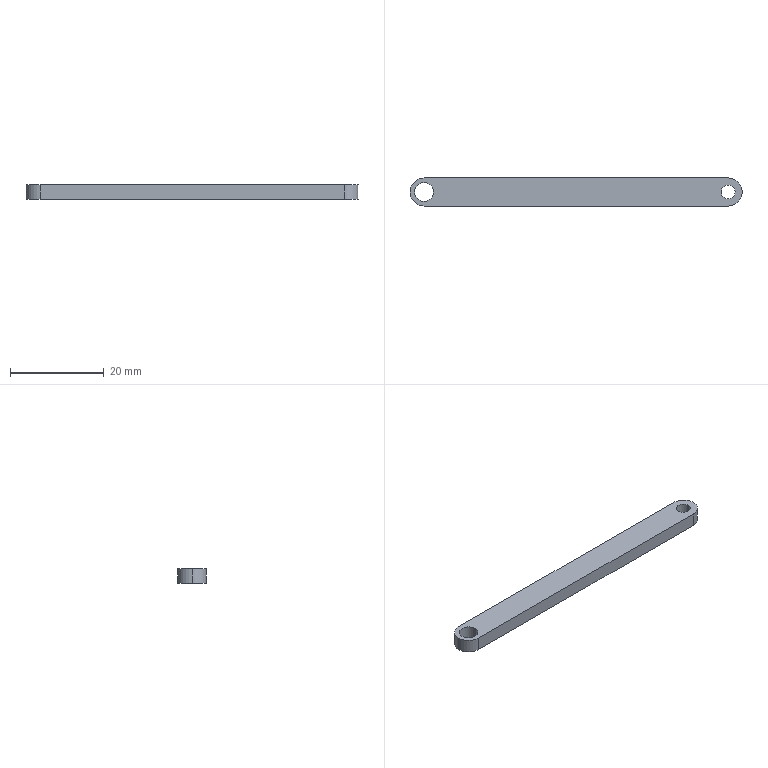Part | SolidWorks | features Extrusion 1, Scale 1 | 1 solid | 11 faces | box 71 x 6 x 3 mm | volume 1196 mm3 | cylinder 7 | plane 4 | commonest cylinder face diameters 6 x3 3 x2 4 x2
STEP:
#1=CARTESIAN_POINT('',(47.312,-1.5,3.));
#2=VERTEX_POINT('',#1);
#3=CARTESIAN_POINT('',(50.312,-1.5,3.));
#4=VERTEX_POINT('',#3);
#5=CARTESIAN_POINT('',(48.812,-1.5,3.));
#6=DIRECTION('',(0.,0.,1.));
#7=DIRECTION('',(1.,0.,0.));
#8=AXIS2_PLACEMENT_3D('',#5,#6,#7);
#9=CIRCLE('',#8,1.5);
#10=EDGE_CURVE('',#2,#4,#9,.T.);
#11=ORIENTED_EDGE('',*,*,#10,.T.);
#12=CARTESIAN_POINT('',(50.312,-1.5,0.));
#13=VERTEX_POINT('',#12);
#14=CARTESIAN_POINT('',(50.312,-1.5,3.));
#15=DIRECTION('',(0.,0.,-1.));
#16=VECTOR('',#15,1000.);
#17=LINE('',#14,#16);
#18=EDGE_CURVE('',#4,#13,#17,.T.);
#19=ORIENTED_EDGE('',*,*,#18,.T.);
#20=CARTESIAN_POINT('',(47.312,-1.5,0.));
#21=VERTEX_POINT('',#20);
#22=CARTESIAN_POINT('',(48.812,-1.5,0.));
#23=DIRECTION('',(0.,0.,1.));
#24=DIRECTION('',(1.,0.,0.));
#25=AXIS2_PLACEMENT_3D('',#22,#23,#24);
#26=CIRCLE('',#25,1.5);
#27=EDGE_CURVE('',#21,#13,#26,.T.);
#28=ORIENTED_EDGE('',*,*,#27,.F.);
#29=CARTESIAN_POINT('',(47.312,-1.5,3.));
#30=DIRECTION('',(0.,0.,-1.));
#31=VECTOR('',#30,1000.);
#32=LINE('',#29,#31);
#33=EDGE_CURVE('',#2,#21,#32,.T.);
#34=ORIENTED_EDGE('',*,*,#33,.F.);
#35=EDGE_LOOP('',(#11,#19,#28,#34));
#36=FACE_OUTER_BOUND('',#35,.T.);
#37=CARTESIAN_POINT('',(48.812,-1.5,3.));
#38=DIRECTION('',(0.,0.,-1.));
#39=DIRECTION('',(-1.,0.,0.));
#40=AXIS2_PLACEMENT_3D('',#37,#38,#39);
#41=CYLINDRICAL_SURFACE('',#40,1.5);
#42=ADVANCED_FACE('',(#36),#41,.F.);
#43=CARTESIAN_POINT('',(-18.188,-1.5,3.));
#44=VERTEX_POINT('',#43);
#45=CARTESIAN_POINT('',(-14.188,-1.5,3.));
#46=VERTEX_POINT('',#45);
#47=CARTESIAN_POINT('',(-16.188,-1.5,3.));
#48=DIRECTION('',(0.,0.,1.));
#49=DIRECTION('',(1.,0.,0.));
#50=AXIS2_PLACEMENT_3D('',#47,#48,#49);
#51=CIRCLE('',#50,2.);
#52=EDGE_CURVE('',#44,#46,#51,.T.);
#53=ORIENTED_EDGE('',*,*,#52,.T.);
#54=CARTESIAN_POINT('',(-14.188,-1.5,0.));
#55=VERTEX_POINT('',#54);
#56=CARTESIAN_POINT('',(-14.188,-1.5,3.));
#57=DIRECTION('',(0.,0.,-1.));
#58=VECTOR('',#57,1000.);
#59=LINE('',#56,#58);
#60=EDGE_CURVE('',#46,#55,#59,.T.);
#61=ORIENTED_EDGE('',*,*,#60,.T.);
#62=CARTESIAN_POINT('',(-18.188,-1.5,0.));
#63=VERTEX_POINT('',#62);
#64=CARTESIAN_POINT('',(-16.188,-1.5,0.));
#65=DIRECTION('',(0.,0.,1.));
#66=DIRECTION('',(1.,0.,0.));
#67=AXIS2_PLACEMENT_3D('',#64,#65,#66);
#68=CIRCLE('',#67,2.);
#69=EDGE_CURVE('',#63,#55,#68,.T.);
#70=ORIENTED_EDGE('',*,*,#69,.F.);
#71=CARTESIAN_POINT('',(-18.188,-1.5,3.));
#72=DIRECTION('',(0.,0.,-1.));
#73=VECTOR('',#72,1000.);
#74=LINE('',#71,#73);
#75=EDGE_CURVE('',#44,#63,#74,.T.);
#76=ORIENTED_EDGE('',*,*,#75,.F.);
#77=EDGE_LOOP('',(#53,#61,#70,#76));
#78=FACE_OUTER_BOUND('',#77,.T.);
#79=CARTESIAN_POINT('',(-16.188,-1.5,3.));
#80=DIRECTION('',(0.,0.,-1.));
#81=DIRECTION('',(-1.,0.,0.));
#82=AXIS2_PLACEMENT_3D('',#79,#80,#81);
#83=CYLINDRICAL_SURFACE('',#82,2.);
#84=ADVANCED_FACE('',(#78),#83,.F.);
#85=CARTESIAN_POINT('',(-19.188,-1.5,3.));
#86=VERTEX_POINT('',#85);
#87=CARTESIAN_POINT('',(-16.188,-4.5,3.));
#88=VERTEX_POINT('',#87);
#89=CARTESIAN_POINT('',(-16.188,-1.5,3.));
#90=DIRECTION('',(0.,0.,1.));
#91=DIRECTION('',(1.,0.,0.));
#92=AXIS2_PLACEMENT_3D('',#89,#90,#91);
#93=CIRCLE('',#92,3.);
#94=EDGE_CURVE('',#86,#88,#93,.T.);
#95=ORIENTED_EDGE('',*,*,#94,.F.);
#96=CARTESIAN_POINT('',(-19.188,-1.5,0.));
#97=VERTEX_POINT('',#96);
#98=CARTESIAN_POINT('',(-19.188,-1.5,3.));
#99=DIRECTION('',(0.,0.,-1.));
#100=VECTOR('',#99,1000.);
#101=LINE('',#98,#100);
#102=EDGE_CURVE('',#86,#97,#101,.T.);
#103=ORIENTED_EDGE('',*,*,#102,.T.);
#104=CARTESIAN_POINT('',(-16.188,-4.5,0.));
#105=VERTEX_POINT('',#104);
#106=CARTESIAN_POINT('',(-16.188,-1.5,0.));
#107=DIRECTION('',(0.,0.,1.));
#108=DIRECTION('',(1.,0.,0.));
#109=AXIS2_PLACEMENT_3D('',#106,#107,#108);
#110=CIRCLE('',#109,3.);
#111=EDGE_CURVE('',#97,#105,#110,.T.);
#112=ORIENTED_EDGE('',*,*,#111,.T.);
#113=CARTESIAN_POINT('',(-16.188,-4.5,3.));
#114=DIRECTION('',(0.,0.,-1.));
#115=VECTOR('',#114,1000.);
#116=LINE('',#113,#115);
#117=EDGE_CURVE('',#88,#105,#116,.T.);
#118=ORIENTED_EDGE('',*,*,#117,.F.);
#119=EDGE_LOOP('',(#95,#103,#112,#118));
#120=FACE_OUTER_BOUND('',#119,.T.);
#121=CARTESIAN_POINT('',(-16.188,-1.5,3.));
#122=DIRECTION('',(0.,0.,-1.));
#123=DIRECTION('',(-1.,0.,0.));
#124=AXIS2_PLACEMENT_3D('',#121,#122,#123);
#125=CYLINDRICAL_SURFACE('',#124,3.);
#126=ADVANCED_FACE('',(#120),#125,.T.);
#127=ORIENTED_EDGE('',*,*,#52,.F.);
#128=CARTESIAN_POINT('',(-16.188,-1.5,3.));
#129=DIRECTION('',(0.,0.,1.));
#130=DIRECTION('',(1.,0.,0.));
#131=AXIS2_PLACEMENT_3D('',#128,#129,#130);
#132=CIRCLE('',#131,2.);
#133=EDGE_CURVE('',#46,#44,#132,.T.);
#134=ORIENTED_EDGE('',*,*,#133,.F.);
#135=EDGE_LOOP('',(#127,#134));
#136=FACE_BOUND('',#135,.T.);
#137=CARTESIAN_POINT('',(-16.188,1.5,3.));
#138=VERTEX_POINT('',#137);
#139=CARTESIAN_POINT('',(-16.188,-1.5,3.));
#140=DIRECTION('',(0.,0.,1.));
#141=DIRECTION('',(1.,0.,0.));
#142=AXIS2_PLACEMENT_3D('',#139,#140,#141);
#143=CIRCLE('',#142,3.);
#144=EDGE_CURVE('',#138,#86,#143,.T.);
#145=ORIENTED_EDGE('',*,*,#144,.T.);
#146=ORIENTED_EDGE('',*,*,#94,.T.);
#147=CARTESIAN_POINT('',(48.812,-4.5,3.));
#148=VERTEX_POINT('',#147);
#149=CARTESIAN_POINT('',(48.812,-4.5,3.));
#150=DIRECTION('',(1.,0.,0.));
#151=VECTOR('',#150,1000.);
#152=LINE('',#149,#151);
#153=EDGE_CURVE('',#88,#148,#152,.T.);
#154=ORIENTED_EDGE('',*,*,#153,.T.);
#155=CARTESIAN_POINT('',(48.812,1.5,3.));
#156=VERTEX_POINT('',#155);
#157=CARTESIAN_POINT('',(48.812,-1.5,3.));
#158=DIRECTION('',(0.,0.,1.));
#159=DIRECTION('',(1.,0.,0.));
#160=AXIS2_PLACEMENT_3D('',#157,#158,#159);
#161=CIRCLE('',#160,3.);
#162=EDGE_CURVE('',#148,#156,#161,.T.);
#163=ORIENTED_EDGE('',*,*,#162,.T.);
#164=CARTESIAN_POINT('',(-16.188,1.5,3.));
#165=DIRECTION('',(-1.,0.,0.));
#166=VECTOR('',#165,1000.);
#167=LINE('',#164,#166);
#168=EDGE_CURVE('',#156,#138,#167,.T.);
#169=ORIENTED_EDGE('',*,*,#168,.T.);
#170=EDGE_LOOP('',(#145,#146,#154,#163,#169));
#171=FACE_OUTER_BOUND('',#170,.T.);
#172=ORIENTED_EDGE('',*,*,#10,.F.);
#173=CARTESIAN_POINT('',(48.812,-1.5,3.));
#174=DIRECTION('',(0.,0.,1.));
#175=DIRECTION('',(1.,0.,0.));
#176=AXIS2_PLACEMENT_3D('',#173,#174,#175);
#177=CIRCLE('',#176,1.5);
#178=EDGE_CURVE('',#4,#2,#177,.T.);
#179=ORIENTED_EDGE('',*,*,#178,.F.);
#180=EDGE_LOOP('',(#172,#179));
#181=FACE_BOUND('',#180,.T.);
#182=CARTESIAN_POINT('',(-16.188,-1.5,3.));
#183=DIRECTION('',(0.,0.,1.));
#184=DIRECTION('',(1.,0.,0.));
#185=AXIS2_PLACEMENT_3D('',#182,#183,#184);
#186=PLANE('',#185);
#187=ADVANCED_FACE('',(#136,#171,#181),#186,.T.);
#188=CARTESIAN_POINT('',(-16.188,1.5,0.));
#189=VERTEX_POINT('',#188);
#190=CARTESIAN_POINT('',(-16.188,-1.5,0.));
#191=DIRECTION('',(0.,0.,1.));
#192=DIRECTION('',(1.,0.,0.));
#193=AXIS2_PLACEMENT_3D('',#190,#191,#192);
#194=CIRCLE('',#193,3.);
#195=EDGE_CURVE('',#189,#97,#194,.T.);
#196=ORIENTED_EDGE('',*,*,#195,.F.);
#197=CARTESIAN_POINT('',(48.812,1.5,0.));
#198=VERTEX_POINT('',#197);
#199=CARTESIAN_POINT('',(-16.188,1.5,0.));
#200=DIRECTION('',(-1.,0.,0.));
#201=VECTOR('',#200,1000.);
#202=LINE('',#199,#201);
#203=EDGE_CURVE('',#198,#189,#202,.T.);
#204=ORIENTED_EDGE('',*,*,#203,.F.);
#205=CARTESIAN_POINT('',(48.812,-4.5,0.));
#206=VERTEX_POINT('',#205);
#207=CARTESIAN_POINT('',(48.812,-1.5,0.));
#208=DIRECTION('',(0.,0.,1.));
#209=DIRECTION('',(1.,0.,0.));
#210=AXIS2_PLACEMENT_3D('',#207,#208,#209);
#211=CIRCLE('',#210,3.);
#212=EDGE_CURVE('',#206,#198,#211,.T.);
#213=ORIENTED_EDGE('',*,*,#212,.F.);
#214=CARTESIAN_POINT('',(48.812,-4.5,0.));
#215=DIRECTION('',(1.,0.,0.));
#216=VECTOR('',#215,1000.);
#217=LINE('',#214,#216);
#218=EDGE_CURVE('',#105,#206,#217,.T.);
#219=ORIENTED_EDGE('',*,*,#218,.F.);
#220=ORIENTED_EDGE('',*,*,#111,.F.);
#221=EDGE_LOOP('',(#196,#204,#213,#219,#220));
#222=FACE_OUTER_BOUND('',#221,.T.);
#223=ORIENTED_EDGE('',*,*,#69,.T.);
#224=CARTESIAN_POINT('',(-16.188,-1.5,0.));
#225=DIRECTION('',(0.,0.,1.));
#226=DIRECTION('',(1.,0.,0.));
#227=AXIS2_PLACEMENT_3D('',#224,#225,#226);
#228=CIRCLE('',#227,2.);
#229=EDGE_CURVE('',#55,#63,#228,.T.);
#230=ORIENTED_EDGE('',*,*,#229,.T.);
#231=EDGE_LOOP('',(#223,#230));
#232=FACE_BOUND('',#231,.T.);
#233=ORIENTED_EDGE('',*,*,#27,.T.);
#234=CARTESIAN_POINT('',(48.812,-1.5,0.));
#235=DIRECTION('',(0.,0.,1.));
#236=DIRECTION('',(1.,0.,0.));
#237=AXIS2_PLACEMENT_3D('',#234,#235,#236);
#238=CIRCLE('',#237,1.5);
#239=EDGE_CURVE('',#13,#21,#238,.T.);
#240=ORIENTED_EDGE('',*,*,#239,.T.);
#241=EDGE_LOOP('',(#233,#240));
#242=FACE_BOUND('',#241,.T.);
#243=CARTESIAN_POINT('',(-16.188,-1.5,0.));
#244=DIRECTION('',(0.,0.,1.));
#245=DIRECTION('',(1.,0.,0.));
#246=AXIS2_PLACEMENT_3D('',#243,#244,#245);
#247=PLANE('',#246);
#248=ADVANCED_FACE('',(#222,#232,#242),#247,.F.);
#249=ORIENTED_EDGE('',*,*,#102,.F.);
#250=ORIENTED_EDGE('',*,*,#144,.F.);
#251=CARTESIAN_POINT('',(-16.188,1.5,3.));
#252=DIRECTION('',(0.,0.,-1.));
#253=VECTOR('',#252,1000.);
#254=LINE('',#251,#253);
#255=EDGE_CURVE('',#138,#189,#254,.T.);
#256=ORIENTED_EDGE('',*,*,#255,.T.);
#257=ORIENTED_EDGE('',*,*,#195,.T.);
#258=EDGE_LOOP('',(#249,#250,#256,#257));
#259=FACE_OUTER_BOUND('',#258,.T.);
#260=CARTESIAN_POINT('',(-16.188,-1.5,3.));
#261=DIRECTION('',(0.,0.,-1.));
#262=DIRECTION('',(-1.,0.,0.));
#263=AXIS2_PLACEMENT_3D('',#260,#261,#262);
#264=CYLINDRICAL_SURFACE('',#263,3.);
#265=ADVANCED_FACE('',(#259),#264,.T.);
#266=ORIENTED_EDGE('',*,*,#218,.T.);
#267=CARTESIAN_POINT('',(48.812,-4.5,3.));
#268=DIRECTION('',(0.,0.,-1.));
#269=VECTOR('',#268,1000.);
#270=LINE('',#267,#269);
#271=EDGE_CURVE('',#148,#206,#270,.T.);
#272=ORIENTED_EDGE('',*,*,#271,.F.);
#273=ORIENTED_EDGE('',*,*,#153,.F.);
#274=ORIENTED_EDGE('',*,*,#117,.T.);
#275=EDGE_LOOP('',(#266,#272,#273,#274));
#276=FACE_OUTER_BOUND('',#275,.T.);
#277=CARTESIAN_POINT('',(48.812,-4.5,3.));
#278=DIRECTION('',(0.,1.,0.));
#279=DIRECTION('',(-1.,0.,0.));
#280=AXIS2_PLACEMENT_3D('',#277,#278,#279);
#281=PLANE('',#280);
#282=ADVANCED_FACE('',(#276),#281,.F.);
#283=ORIENTED_EDGE('',*,*,#212,.T.);
#284=CARTESIAN_POINT('',(48.812,1.5,3.));
#285=DIRECTION('',(0.,0.,-1.));
#286=VECTOR('',#285,1000.);
#287=LINE('',#284,#286);
#288=EDGE_CURVE('',#156,#198,#287,.T.);
#289=ORIENTED_EDGE('',*,*,#288,.F.);
#290=ORIENTED_EDGE('',*,*,#162,.F.);
#291=ORIENTED_EDGE('',*,*,#271,.T.);
#292=EDGE_LOOP('',(#283,#289,#290,#291));
#293=FACE_OUTER_BOUND('',#292,.T.);
#294=CARTESIAN_POINT('',(48.812,-1.5,3.));
#295=DIRECTION('',(0.,0.,-1.));
#296=DIRECTION('',(-1.,0.,0.));
#297=AXIS2_PLACEMENT_3D('',#294,#295,#296);
#298=CYLINDRICAL_SURFACE('',#297,3.);
#299=ADVANCED_FACE('',(#293),#298,.T.);
#300=ORIENTED_EDGE('',*,*,#203,.T.);
#301=ORIENTED_EDGE('',*,*,#255,.F.);
#302=ORIENTED_EDGE('',*,*,#168,.F.);
#303=ORIENTED_EDGE('',*,*,#288,.T.);
#304=EDGE_LOOP('',(#300,#301,#302,#303));
#305=FACE_OUTER_BOUND('',#304,.T.);
#306=CARTESIAN_POINT('',(-16.188,1.5,3.));
#307=DIRECTION('',(0.,-1.,0.));
#308=DIRECTION('',(0.,0.,-1.));
#309=AXIS2_PLACEMENT_3D('',#306,#307,#308);
#310=PLANE('',#309);
#311=ADVANCED_FACE('',(#305),#310,.F.);
#312=ORIENTED_EDGE('',*,*,#60,.F.);
#313=ORIENTED_EDGE('',*,*,#133,.T.);
#314=ORIENTED_EDGE('',*,*,#75,.T.);
#315=ORIENTED_EDGE('',*,*,#229,.F.);
#316=EDGE_LOOP('',(#312,#313,#314,#315));
#317=FACE_OUTER_BOUND('',#316,.T.);
#318=CARTESIAN_POINT('',(-16.188,-1.5,3.));
#319=DIRECTION('',(0.,0.,-1.));
#320=DIRECTION('',(-1.,0.,0.));
#321=AXIS2_PLACEMENT_3D('',#318,#319,#320);
#322=CYLINDRICAL_SURFACE('',#321,2.);
#323=ADVANCED_FACE('',(#317),#322,.F.);
#324=ORIENTED_EDGE('',*,*,#18,.F.);
#325=ORIENTED_EDGE('',*,*,#178,.T.);
#326=ORIENTED_EDGE('',*,*,#33,.T.);
#327=ORIENTED_EDGE('',*,*,#239,.F.);
#328=EDGE_LOOP('',(#324,#325,#326,#327));
#329=FACE_OUTER_BOUND('',#328,.T.);
#330=CARTESIAN_POINT('',(48.812,-1.5,3.));
#331=DIRECTION('',(0.,0.,-1.));
#332=DIRECTION('',(-1.,0.,0.));
#333=AXIS2_PLACEMENT_3D('',#330,#331,#332);
#334=CYLINDRICAL_SURFACE('',#333,1.5);
#335=ADVANCED_FACE('',(#329),#334,.F.);
#336=CLOSED_SHELL('',(#42,#84,#126,#187,#248,#265,#282,#299,#311,#323,#335));
#337=MANIFOLD_SOLID_BREP('',#336);
#338=CARTESIAN_POINT('',(0.,0.,0.));
#339=DIRECTION('',(0.,0.,1.));
#340=DIRECTION('',(1.,0.,0.));
#341=AXIS2_PLACEMENT_3D('',#338,#339,#340);
#342=(LENGTH_UNIT()NAMED_UNIT(*)SI_UNIT(.MILLI.,.METRE.));
#343=UNCERTAINTY_MEASURE_WITH_UNIT(LENGTH_MEASURE(0.00001),#342,'','');
#344=(NAMED_UNIT(*)PLANE_ANGLE_UNIT()SI_UNIT($,.RADIAN.));
#345=(NAMED_UNIT(*)SI_UNIT($,.STERADIAN.)SOLID_ANGLE_UNIT());
#346=(GEOMETRIC_REPRESENTATION_CONTEXT(3)GLOBAL_UNCERTAINTY_ASSIGNED_CONTEXT((#343))GLOBAL_UNIT_ASSIGNED_CONTEXT((#342,#344,#345))REPRESENTATION_CONTEXT('',''));
#347=ADVANCED_BREP_SHAPE_REPRESENTATION('',(#337,#341),#346);